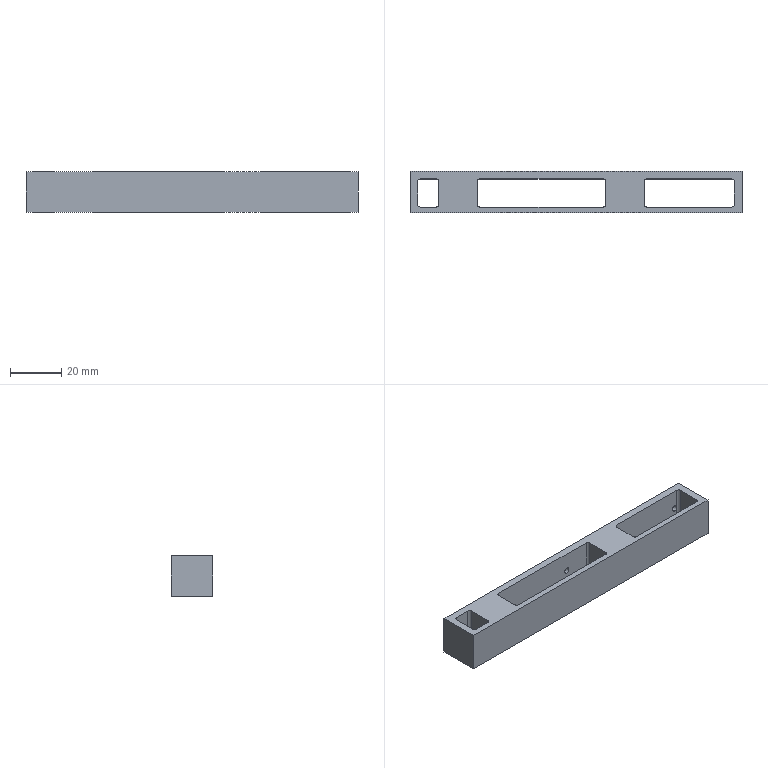NC program | NX | posted with a generic post | part box 130 x 16.2 x 16 mm
Whole program:
N10 G17 G21 G94 G90
(FLOOR_WALL_COPY , TOOL : D63)
N12 T01 M6
N14 G54
N16 G17 G0 G90 X-99.5 Y0. B0. C0. S6500 M3
N18 G43 Z30. H1
N20 Z6.
N22 G94 G1 Z3. F1250.
N24 X-96.5
N26 X96.5
N28 X99.5
N30 Z6.
N32 G0 Z30.
N34 X-99.5
N36 Z5.
N38 G1 Z2.
N40 X-96.5
N42 X96.5
N44 X99.5
N46 Z5.
N48 G0 Z30.
N50 X-99.5
N52 Z4.
N54 G1 Z1.
N56 X-96.5
N58 X96.5
N60 X99.5
N62 Z4.
N64 G0 Z30.
N66 X-99.5
N68 Z3.
N70 G1 Z0.
N72 X-96.5
N74 X96.5
N76 X99.5
N78 Z3.
N80 G0 Z30.
N82 M5
(PLANAR_MILL_COPY , TOOL : D6A45)
N84 T07 M6
N86 G54
N88 G17 G0 G90 X-45.117 Y-4.643 B0. C0. S9500 M3
N90 G43 Z30. H7
N92 Z0.5
N94 G94 G1 Z-1. F1250.
N96 G3 X-44.351 Y-5. R1.
N98 G1 X-27.702
N100 X-27.637 Y-5.013
N102 X-27.589 Y-4.965
N104 X-27.602 Y-4.9
N106 Y4.1
N108 X-27.589 Y4.165
N110 X-27.637 Y4.213
N112 X-27.702 Y4.2
N114 X-61.
N116 X-61.065 Y4.213
N118 X-61.113 Y4.165
N120 X-61.1 Y4.1
N122 Y-4.9
N124 X-61.113 Y-4.965
N126 X-61.065 Y-5.013
N128 X-61. Y-5.
N130 X-44.351
N132 G3 X-43.585 Y-4.643 R1.
N134 G1 Z0.5
N136 G0 Z30.
N138 X-0.766 Y9.357
N140 Z0.5
N142 G1 Z-1.
N144 G3 X0. Y9. R1.
N146 G1 X65.
N148 G2 X65.9 Y8.1 R0.9
N150 G1 Y-8.1
N152 G2 X65. Y-9. R0.9
N154 G1 X-65.
N156 G2 X-65.9 Y-8.1 R0.9
N158 G1 Y8.1
N160 G2 X-65. Y9. R0.9
N162 G1 X0.
N164 G3 X0.766 Y9.357 R1.
N166 G1 Z0.5
N168 G0 Z30.
N170 X14.269 Y3.843
N172 Z0.5
N174 G1 Z-1.
N176 G3 X13.503 Y4.2 R1.
N178 G1 X-10.702
N180 X-10.767 Y4.213
N182 X-10.814 Y4.165
N184 X-10.802 Y4.1
N186 Y-4.9
N188 X-10.814 Y-4.965
N190 X-10.767 Y-5.013
N192 X-10.702 Y-5.
N194 X37.708
N196 X37.773 Y-5.013
N198 X37.821 Y-4.965
N200 X37.808 Y-4.9
N202 Y4.1
N204 X37.821 Y4.165
N206 X37.773 Y4.213
N208 X37.708 Y4.2
N210 X13.503
N212 G3 X12.737 Y3.843 R1.
N214 G1 Z0.5
N216 G0 Z30.
N218 X60.743 Y-1.166
N220 Z0.5
N222 G1 Z-1.
N224 G3 X61.1 Y-0.4 R1.
N226 G1 Y4.1
N228 X61.113 Y4.165
N230 X61.065 Y4.213
N232 X61. Y4.2
N234 X54.708
N236 X54.643 Y4.213
N238 X54.596 Y4.165
N240 X54.608 Y4.1
N242 Y-4.9
N244 X54.596 Y-4.965
N246 X54.643 Y-5.013
N248 X54.708 Y-5.
N250 X61.
N252 X61.065 Y-5.013
N254 X61.113 Y-4.965
N256 X61.1 Y-4.9
N258 Y-0.4
N260 G3 X60.743 Y0.366 R1.
N262 G1 Z0.5
N264 G0 Z30.
N266 M5
N268 M2